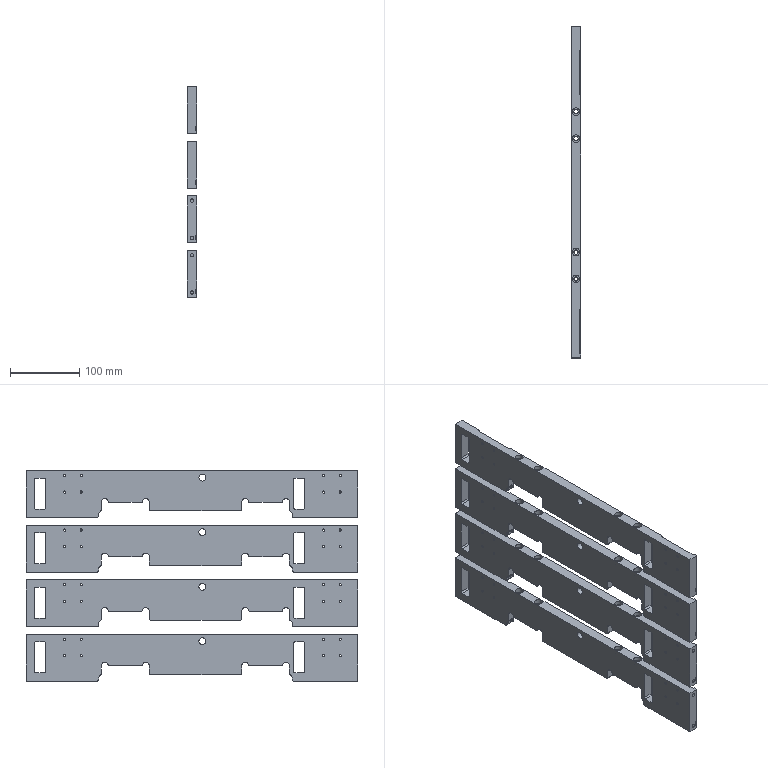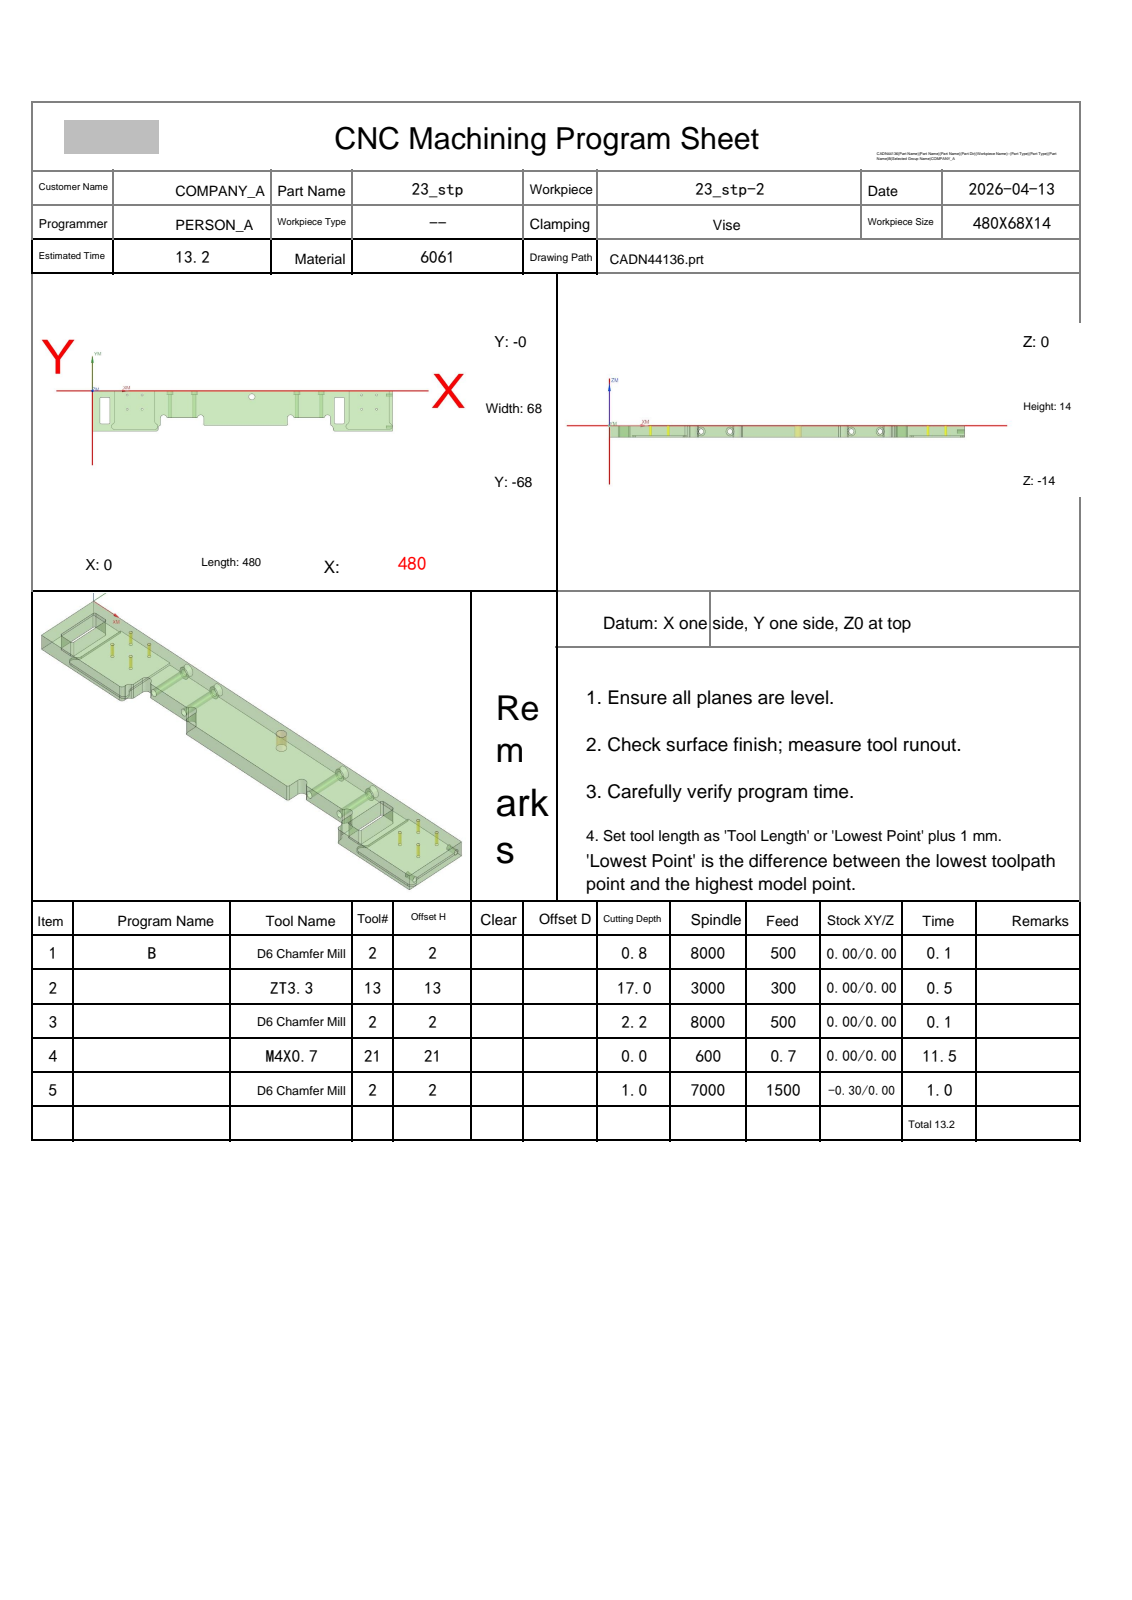NC program | NX | posted by the shop | part box 14 x 480 x 305 mm
Whole program:
%
O0001
(Machine time: 14.31 MIN)
(===Total Tool:3===)
(T2=D6 Chamfer Mill   D=6.   R=0.   D-  H02 Z=-2.15 )
(T13=ZT3.3  D=3.3  DR_a=118 D-  H13 Z=-17.  )
(T21=M4X0.7 D=3.3  DR_a=180 D-  H21 Z=0.    )
G80 G90 G17 G49 G40
G91 G28 Z0
M01
N1 T02 M06
(D6 Chamfer Mill  D=6. R=0. H=02 ce=0.00 di=0.00)
G00 G90 G54 X79.5 Y-7. M03 S8000
G43 H02 Z20.
M08
G98 G81 X79.5 Y-7. Z-.8 R1. F500.
X55.5
Y-31.
X79.5
X430.5
Y-7.
X454.5
Y-31.
G80
G00 Z20.
G91 G28 Z0.0
M05
M09
G91 G28 Z0.0
M01
N2 T13 M06
(ZT3.3 D=3.3 DR_a=118 H=13)
G00 G90 G54 X79.5 Y-7. M03 S3000
G43 H13 Z20.
M08
G98 G83 X79.5 Y-7. Z-17. R1. F300. Q2.
X55.5
Y-31.
X79.5
X430.5
Y-7.
X454.5
Y-31.
G80
G00 Z20.
G91 G28 Z0.0
M05
M09
G91 G28 Z0.0
M01
N3 T02 M06
(D6 Chamfer Mill  D=6. R=0. H=02 ce=0.00 di=0.00)
G00 G90 G54 X79.5 Y-7. M03 S8000
G43 H02 Z20.
M08
G98 G81 X79.5 Y-7. Z-2.15 R3. F500.
X55.5
Y-31.
X79.5
X430.5
Y-7.
X454.5
Y-31.
G80
G00 Z20.
G91 G28 Z0.0
M05
M09
G91 G28 Z0.0
M01
N4 T21 M06
(M4X0.7 D=3.3 DR_a=180 H=21)
G00 G90 G54 X79.5 Y-7. M03 S600
G43 H21 Z20.
M08
G95
G98 G84 X79.5 Y-7. Z0.0 R1. F.7 Q4.
X55.5
Y-31.
X79.5
X430.5
Y-7.
X454.5
Y-31.
G80
G94
G00 Z20.
G91 G28 Z0.0
M05
M09
G91 G28 Z0.0
M01
N5 T02 M06
(D6 Chamfer Mill  D=6. R=0. H=02 ce=-0.30 di=0.00)
G00 G90 G54 X18.428 Y-55.05 M03 S7000
G43 H02 Z20.
M08
Z2.5
G01 X26.088 Z-.288 F1500.
X26.319 Y-55.013 Z-.373
X26.539 Y-54.936 Z-.458
X26.742 Y-54.821 Z-.543
X26.921 Y-54.671 Z-.628
X27.071 Y-54.492 Z-.713
X27.186 Y-54.289 Z-.798
X27.263 Y-54.069 Z-.883
X27.3 Y-53.838 Z-.968
Y-53.75 Z-1.
Y-12.75
G03 X26. Y-11.45 I-1.3 J0.0
G01 X14.
G03 X12.7 Y-12.75 I0.0 J-1.3
G01 Y-53.75
G03 X14. Y-55.05 I1.3 J0.0
G01 X26.
G03 X27.3 Y-53.75 I0.0 J1.3
G01 Y-53.25
Z1.5
G00 Z20.
X116.554 Y-42.015
Z2.5
G01 X116.207 Y-41.768 Z2.345
X115.814 Y-41.546 Z2.18
X115.399 Y-41.367 Z2.016
X114.969 Y-41.232 Z1.852
X114.526 Y-41.143 Z1.688
X114.076 Y-41.101 Z1.523
X113.625 Y-41.106 Z1.359
X113.177 Y-41.158 Z1.195
X112.736 Y-41.257 Z1.03
X112.309 Y-41.402 Z.866
X111.898 Y-41.591 Z.702
X111.51 Y-41.822 Z.537
X111.149 Y-42.092 Z.373
X110.817 Y-42.398 Z.209
X110.52 Y-42.738 Z.044
X110.259 Y-43.106 Z-.12
X110.039 Y-43.5 Z-.284
X109.861 Y-43.915 Z-.449
X109.728 Y-44.347 Z-.613
X109.64 Y-44.79 Z-.777
X109.6 Y-45.239 Z-.942
Y-45.4 Z-1.
Y-56.722
G02 X108.096 Y-59.143 I-2.7 J0.0
G03 X105.7 Y-62.999 I1.904 J-3.855
G01 Y-65.
G02 X102. Y-68.7 I-3.7 J0.0
G01 X.3
G02 X-.7 Y-67.7 I0.0 J1.
G01 Y-.3
G02 X.3 Y.7 I1. J0.0
G01 X479.7
G02 X480.7 Y-.3 I0.0 J-1.
G01 Y-67.7
G02 X479.7 Y-68.7 I-1. J0.0
G01 X388.
G02 X384.3 Y-65. I0.0 J3.7
G01 Y-62.999
G03 X381.904 Y-59.143 I-4.3 J0.0
G02 X380.4 Y-56.722 I1.196 J2.421
G01 Y-45.4
G03 X376.1 Y-41.1 I-4.3 J0.0
X371.916 Y-44.408 I0.0 J-4.3
G02 X369.775 Y-46.1 I-2.141 J.508
G01 X323.225
G02 X321.084 Y-44.408 I0.0 J2.2
G03 X316.9 Y-41.1 I-4.184 J-.992
X312.6 Y-45.4 I0.0 J-4.3
G01 Y-56.4
G02 X309.9 Y-59.1 I-2.7 J0.0
G01 X180.1
G02 X177.4 Y-56.4 I0.0 J2.7
G01 Y-45.4
G03 X173.1 Y-41.1 I-4.3 J0.0
X168.916 Y-44.408 I0.0 J-4.3
G02 X166.775 Y-46.1 I-2.141 J.508
G01 X120.225
G02 X118.084 Y-44.408 I0.0 J2.2
G03 X113.9 Y-41.1 I-4.184 J-.992
X109.6 Y-45.4 I0.0 J-4.3
G01 Y-45.9
Z1.5
G00 Z20.
X258.386 Y-12.654
Z2.5
G01 X258.394 Y-12.645 Z2.495
X258.644 Y-12.289 Z2.337
X258.804 Y-12.011 Z2.22
X258.988 Y-11.617 Z2.062
X259.13 Y-11.207 Z1.904
X259.231 Y-10.784 Z1.746
X259.288 Y-10.354 Z1.588
X259.302 Y-9.92 Z1.43
X259.272 Y-9.486 Z1.272
X259.199 Y-9.058 Z1.114
X259.082 Y-8.64 Z.956
X258.924 Y-8.235 Z.797
X258.727 Y-7.849 Z.639
X258.491 Y-7.484 Z.481
X258.219 Y-7.145 Z.323
X257.915 Y-6.835 Z.165
X257.581 Y-6.557 Z.007
X257.221 Y-6.314 Z-.151
X256.838 Y-6.109 Z-.309
X256.436 Y-5.944 Z-.467
X256.02 Y-5.82 Z-.625
X255.593 Y-5.738 Z-.783
X255.161 Y-5.7 Z-.942
X255. Z-1.
G03 X250.7 Y-10. I0.0 J-4.3
X255. Y-14.3 I4.3 J0.0
X259.3 Y-10. I0.0 J4.3
X255. Y-5.7 I-4.3 J0.0
X254.501 Y-5.729 I0.0 J-4.3
G01 Z1.5
G00 Z20.
X393.428 Y-55.05
Z2.5
G01 X401.088 Z-.288
X401.319 Y-55.013 Z-.373
X401.539 Y-54.936 Z-.458
X401.742 Y-54.821 Z-.543
X401.921 Y-54.671 Z-.628
X402.071 Y-54.492 Z-.713
X402.186 Y-54.289 Z-.798
X402.263 Y-54.069 Z-.883
X402.3 Y-53.838 Z-.968
Y-53.75 Z-1.
Y-12.75
G03 X401. Y-11.45 I-1.3 J0.0
G01 X389.
G03 X387.7 Y-12.75 I0.0 J-1.3
G01 Y-53.75
G03 X389. Y-55.05 I1.3 J0.0
G01 X401.
G03 X402.3 Y-53.75 I0.0 J1.3
G01 Y-53.25
Z1.5
G00 Z20.
M05
M09
G91 G28 Z0.0
G91 G28 Y0.0
M30
%